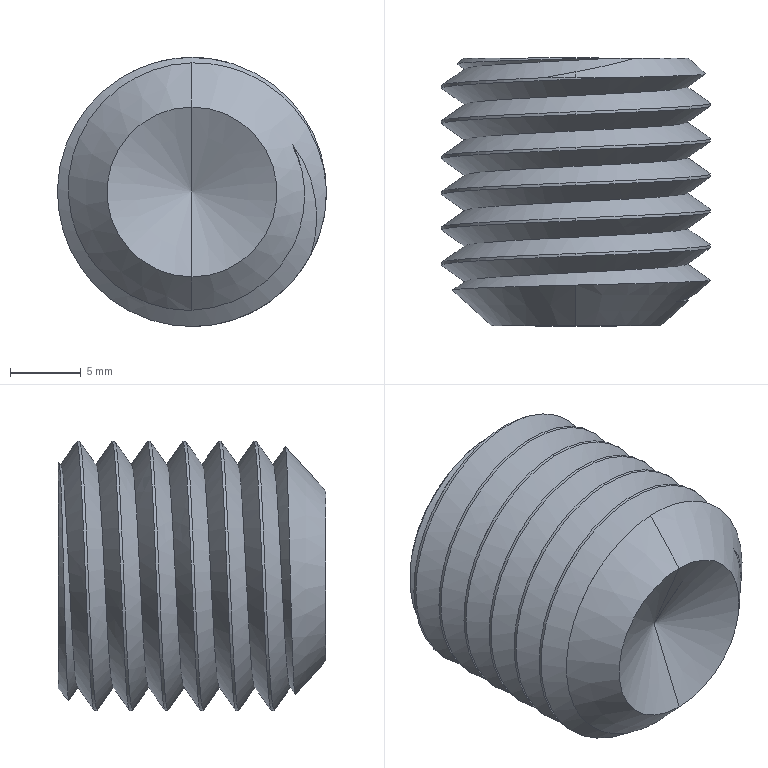Part | STEP file | Plug 3_4'' | 1 solid | 32 faces | box 19 x 18.901 x 19 mm | volume 3394 mm3 | cylinder 13 | cone 10 | plane 7 | spline 2 | commonest cylinder face diameters 19 x13